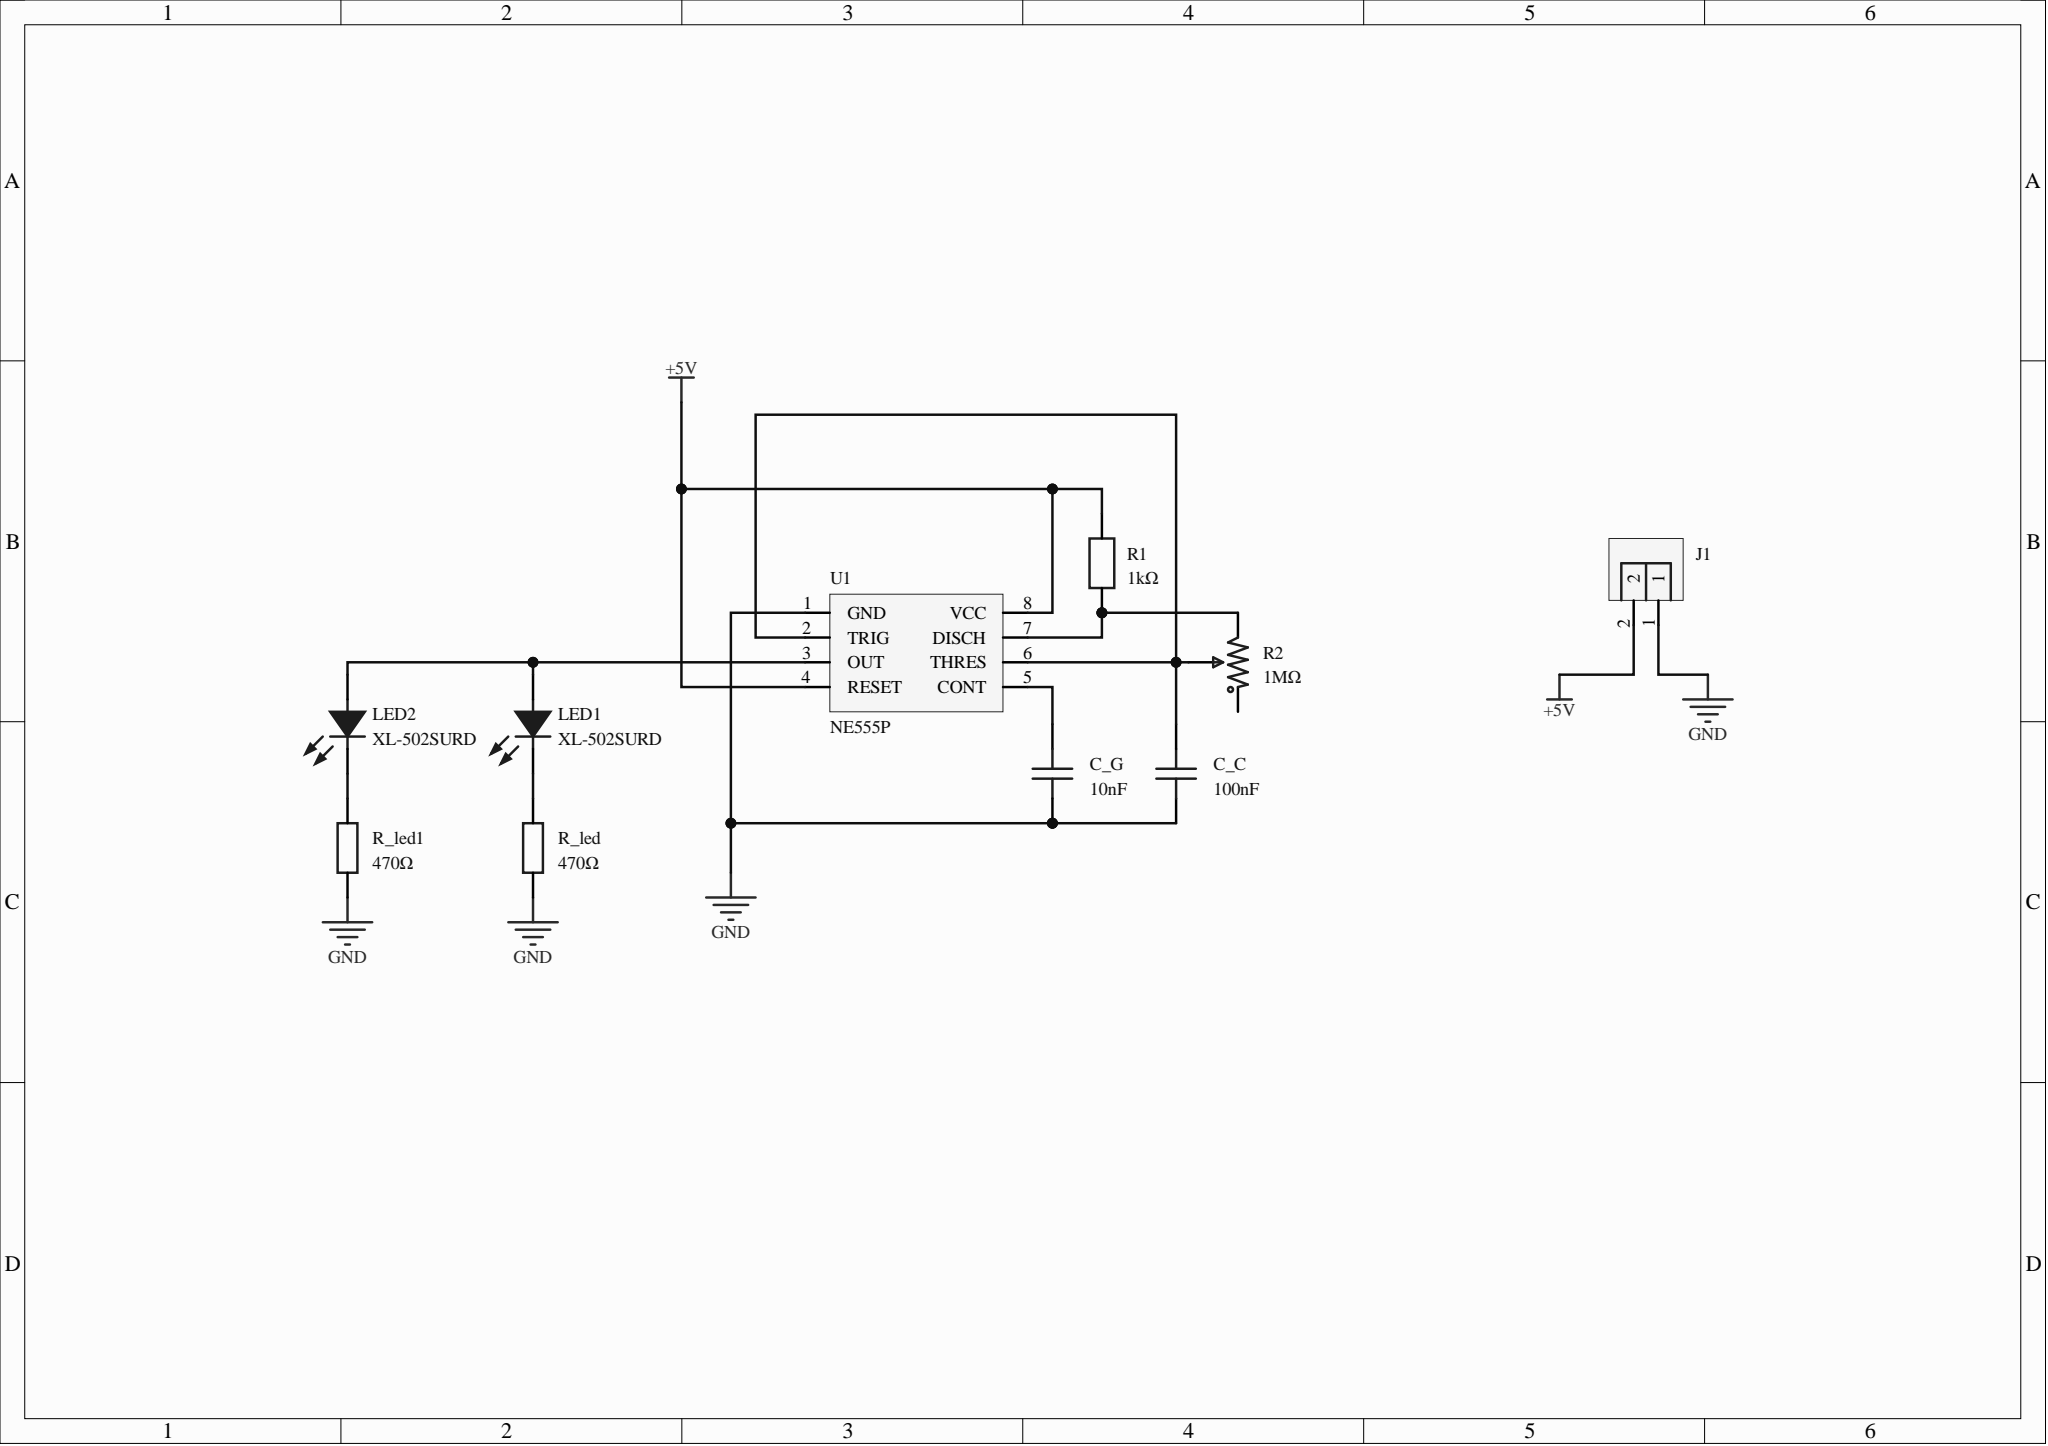Circuit board | Altium Designer | 10 parts | 8 nets
Bill of materials:
Comment,Description,Designator,Footprint,LibRef,Quantity
"100nF","Capacitance: 100nF; tolerance: ±20%; rated voltage: 50V; temperature coefficient: Y5V;","C_C","CAP-TH_L5.0-W2.5-P5.00-D1.0","CC1H104MC1FD3F6C10MF","1"
"10nF","Capacitance: 10nF; tolerance: ±20%; rated voltage: 50V; temperature coefficient: Y5U;","C_G","CAP-TH_L5.5-W3.0-P5.00-D0.6","DCT103M22Y5UF6FJ5A0","1"
"","","J1","HDR-TH_2P-P2.54-V-M-1","HDR-M_2.54_1x2P","1"
"XL-502SURD","","LED1, LED2","LED-TH_BD5.9-P2.54-RD_RED","XL-502SURD","2"
"1kΩ","Resistor type: metal film resistor; resistance: 1kΩ; tolerance: ±1%; power: 250mW; temperature coefficient: ±100ppm/?;","R1","RES-TH_BD2.7-L6.2-P10.20-D0.4","MF1/4W-1K±1%-ST52","1"
"1MΩ","Resistance: 1MΩ; tolerance: ±25%; power: 100mW;","R2","RES-ADJ-TH_RM063-103","RM063-105(1M)","1"
"470Ω","Resistor type: metal film resistor; resistance: 470Ω; tolerance: ±1%; power: 500mW; temperature coefficient: ±100ppm/?;","R_led, R_led1","RES-TH_BD2.3-L6.5-P10.50-D0.5","MF1/2WS-470Ω±1% T","2"
"NE555P","These devices are precision timing circuits that generate accurate time delays or oscillations. In delay or monostable mode, the timing interval is controlled by a single external resistor and capacitor network. In astable mode, the frequency and duty cycle can be controlled separately by two external resistors and one external capacitor.","U1","DIP-8_L9.8-W6.6-P2.54-LS7.6-BL","NE555P","1"
Netlist (Protel format):
[
C_C
CAP-TH_L5.0-W2.5-P5.00-D1.0
100nF



]
[
C_G
CAP-TH_L5.5-W3.0-P5.00-D0.6
10nF



]
[
J1
HDR-TH_2P-P2.54-V-M-1




]
[
LED1
LED-TH_BD5.9-P2.54-RD_RED
XL-502SURD



]
[
LED2
LED-TH_BD5.9-P2.54-RD_RED
XL-502SURD



]
[
R1
RES-TH_BD2.7-L6.2-P10.20-D0.4
1kΩ



]
[
R2
RES-ADJ-TH_RM063-103
1MΩ



]
[
R_led
RES-TH_BD2.3-L6.5-P10.50-D0.5
470Ω



]
[
R_led1
RES-TH_BD2.3-L6.5-P10.50-D0.5
470Ω



]
[
U1
DIP-8_L9.8-W6.6-P2.54-LS7.6-BL
NE555P



]
(
NetR1_1
R1-1
R2-3
U1-7
)
(
NetLED2_1
LED2-1
R_led1-2
)
(
NetLED1_2
LED1-2
LED2-2
U1-3
)
(
NetLED1_1
LED1-1
R_led-2
)
(
NetC_G_2
C_G-2
U1-5
)
(
NetC_C_2
C_C-2
R2-2
U1-2
U1-6
)
(
GND
C_C-1
C_G-1
J1-1
R_led-1
R_led1-1
U1-1
)
(
+5V
J1-2
R1-2
U1-4
U1-8
)